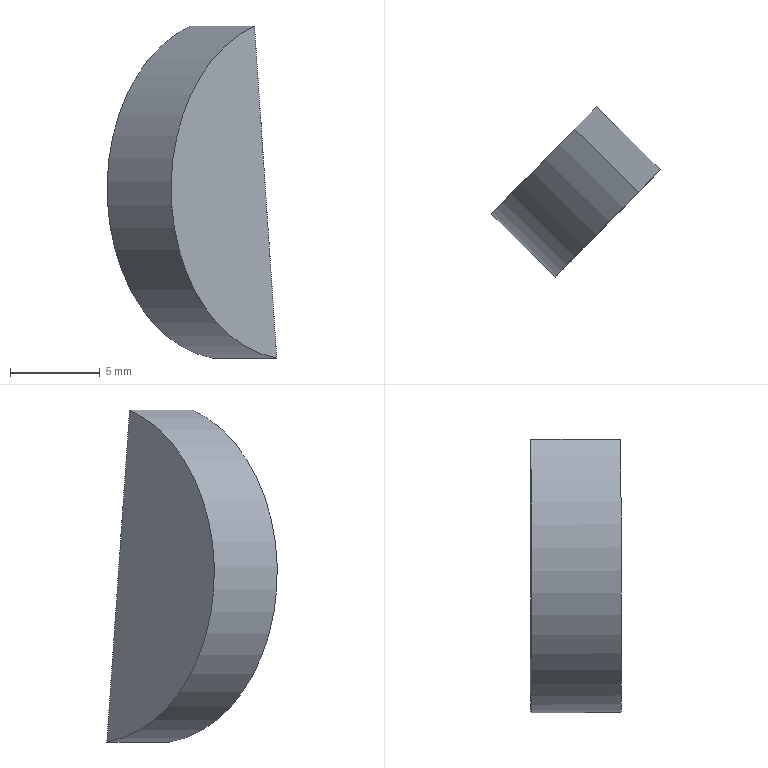Part | SolidWorks | features BaseBody 1 | 1 solid | 4 faces | box 9.451 x 9.493 x 18.489 mm | volume 520.235 mm3 | plane 3 | cylinder 1 | commonest cylinder face diameters 19 x1
STEP:
#1=CARTESIAN_POINT('',(-32.36,-41.355,102.214));
#2=VERTEX_POINT('',#1);
#3=CARTESIAN_POINT('',(-33.603,-42.62,120.704));
#4=VERTEX_POINT('',#3);
#5=CARTESIAN_POINT('',(-31.587,-40.568,111.65));
#6=DIRECTION('',(-0.7133,0.7009,0.));
#7=DIRECTION('',(0.06692,0.0681,-0.9954));
#8=AXIS2_PLACEMENT_3D('',#5,#6,#7);
#9=CIRCLE('',#8,9.5);
#10=EDGE_CURVE('',#2,#4,#9,.T.);
#11=ORIENTED_EDGE('',*,*,#10,.F.);
#12=CARTESIAN_POINT('',(-33.603,-42.62,120.704));
#13=DIRECTION('',(0.06692,0.0681,-0.9954));
#14=VECTOR('',#13,1000.);
#15=LINE('',#12,#14);
#16=EDGE_CURVE('',#4,#2,#15,.T.);
#17=ORIENTED_EDGE('',*,*,#16,.F.);
#18=EDGE_LOOP('',(#11,#17));
#19=FACE_OUTER_BOUND('',#18,.T.);
#20=CARTESIAN_POINT('',(-31.587,-40.568,111.65));
#21=DIRECTION('',(-0.7133,0.7009,0.));
#22=DIRECTION('',(0.,0.,1.));
#23=AXIS2_PLACEMENT_3D('',#20,#21,#22);
#24=PLANE('',#23);
#25=ADVANCED_FACE('',(#19),#24,.F.);
#26=CARTESIAN_POINT('',(-35.927,-37.851,102.214));
#27=VERTEX_POINT('',#26);
#28=CARTESIAN_POINT('',(-37.17,-39.115,120.704));
#29=VERTEX_POINT('',#28);
#30=CARTESIAN_POINT('',(-35.153,-37.063,111.65));
#31=DIRECTION('',(-0.7133,0.7009,0.));
#32=DIRECTION('',(0.06692,0.0681,-0.9954));
#33=AXIS2_PLACEMENT_3D('',#30,#31,#32);
#34=CIRCLE('',#33,9.5);
#35=EDGE_CURVE('',#27,#29,#34,.T.);
#36=ORIENTED_EDGE('',*,*,#35,.T.);
#37=CARTESIAN_POINT('',(-37.17,-39.115,120.704));
#38=DIRECTION('',(0.06692,0.0681,-0.9954));
#39=VECTOR('',#38,1000.);
#40=LINE('',#37,#39);
#41=EDGE_CURVE('',#29,#27,#40,.T.);
#42=ORIENTED_EDGE('',*,*,#41,.T.);
#43=EDGE_LOOP('',(#36,#42));
#44=FACE_OUTER_BOUND('',#43,.T.);
#45=CARTESIAN_POINT('',(-35.153,-37.063,111.65));
#46=DIRECTION('',(-0.7133,0.7009,0.));
#47=DIRECTION('',(0.,0.,1.));
#48=AXIS2_PLACEMENT_3D('',#45,#46,#47);
#49=PLANE('',#48);
#50=ADVANCED_FACE('',(#44),#49,.T.);
#51=ORIENTED_EDGE('',*,*,#16,.T.);
#52=CARTESIAN_POINT('',(-35.927,-37.851,102.214));
#53=DIRECTION('',(-0.7133,0.7009,0.));
#54=VECTOR('',#53,1000.);
#55=LINE('',#52,#54);
#56=EDGE_CURVE('',#2,#27,#55,.T.);
#57=ORIENTED_EDGE('',*,*,#56,.T.);
#58=ORIENTED_EDGE('',*,*,#41,.F.);
#59=CARTESIAN_POINT('',(-37.17,-39.115,120.704));
#60=DIRECTION('',(0.7133,-0.7009,0.));
#61=VECTOR('',#60,1000.);
#62=LINE('',#59,#61);
#63=EDGE_CURVE('',#29,#4,#62,.T.);
#64=ORIENTED_EDGE('',*,*,#63,.T.);
#65=EDGE_LOOP('',(#51,#57,#58,#64));
#66=FACE_OUTER_BOUND('',#65,.T.);
#67=CARTESIAN_POINT('',(-37.17,-39.115,120.704));
#68=DIRECTION('',(-0.6977,-0.71,-0.09548));
#69=DIRECTION('',(-0.7133,0.7009,0.));
#70=AXIS2_PLACEMENT_3D('',#67,#68,#69);
#71=PLANE('',#70);
#72=ADVANCED_FACE('',(#66),#71,.F.);
#73=ORIENTED_EDGE('',*,*,#10,.T.);
#74=ORIENTED_EDGE('',*,*,#63,.F.);
#75=ORIENTED_EDGE('',*,*,#35,.F.);
#76=ORIENTED_EDGE('',*,*,#56,.F.);
#77=EDGE_LOOP('',(#73,#74,#75,#76));
#78=FACE_OUTER_BOUND('',#77,.T.);
#79=CARTESIAN_POINT('',(-35.153,-37.063,111.65));
#80=DIRECTION('',(0.7133,-0.7009,0.));
#81=DIRECTION('',(-0.06692,-0.0681,0.9954));
#82=AXIS2_PLACEMENT_3D('',#79,#80,#81);
#83=CYLINDRICAL_SURFACE('',#82,9.5);
#84=ADVANCED_FACE('',(#78),#83,.T.);
#85=CLOSED_SHELL('',(#25,#50,#72,#84));
#86=MANIFOLD_SOLID_BREP('',#85);
#87=CARTESIAN_POINT('',(0.,0.,0.));
#88=DIRECTION('',(0.,0.,1.));
#89=DIRECTION('',(1.,0.,0.));
#90=AXIS2_PLACEMENT_3D('',#87,#88,#89);
#91=(LENGTH_UNIT()NAMED_UNIT(*)SI_UNIT(.MILLI.,.METRE.));
#92=UNCERTAINTY_MEASURE_WITH_UNIT(LENGTH_MEASURE(0.00001),#91,'','');
#93=(NAMED_UNIT(*)PLANE_ANGLE_UNIT()SI_UNIT($,.RADIAN.));
#94=(NAMED_UNIT(*)SI_UNIT($,.STERADIAN.)SOLID_ANGLE_UNIT());
#95=(GEOMETRIC_REPRESENTATION_CONTEXT(3)GLOBAL_UNCERTAINTY_ASSIGNED_CONTEXT((#92))GLOBAL_UNIT_ASSIGNED_CONTEXT((#91,#93,#94))REPRESENTATION_CONTEXT('',''));
#96=ADVANCED_BREP_SHAPE_REPRESENTATION('',(#86,#90),#95);